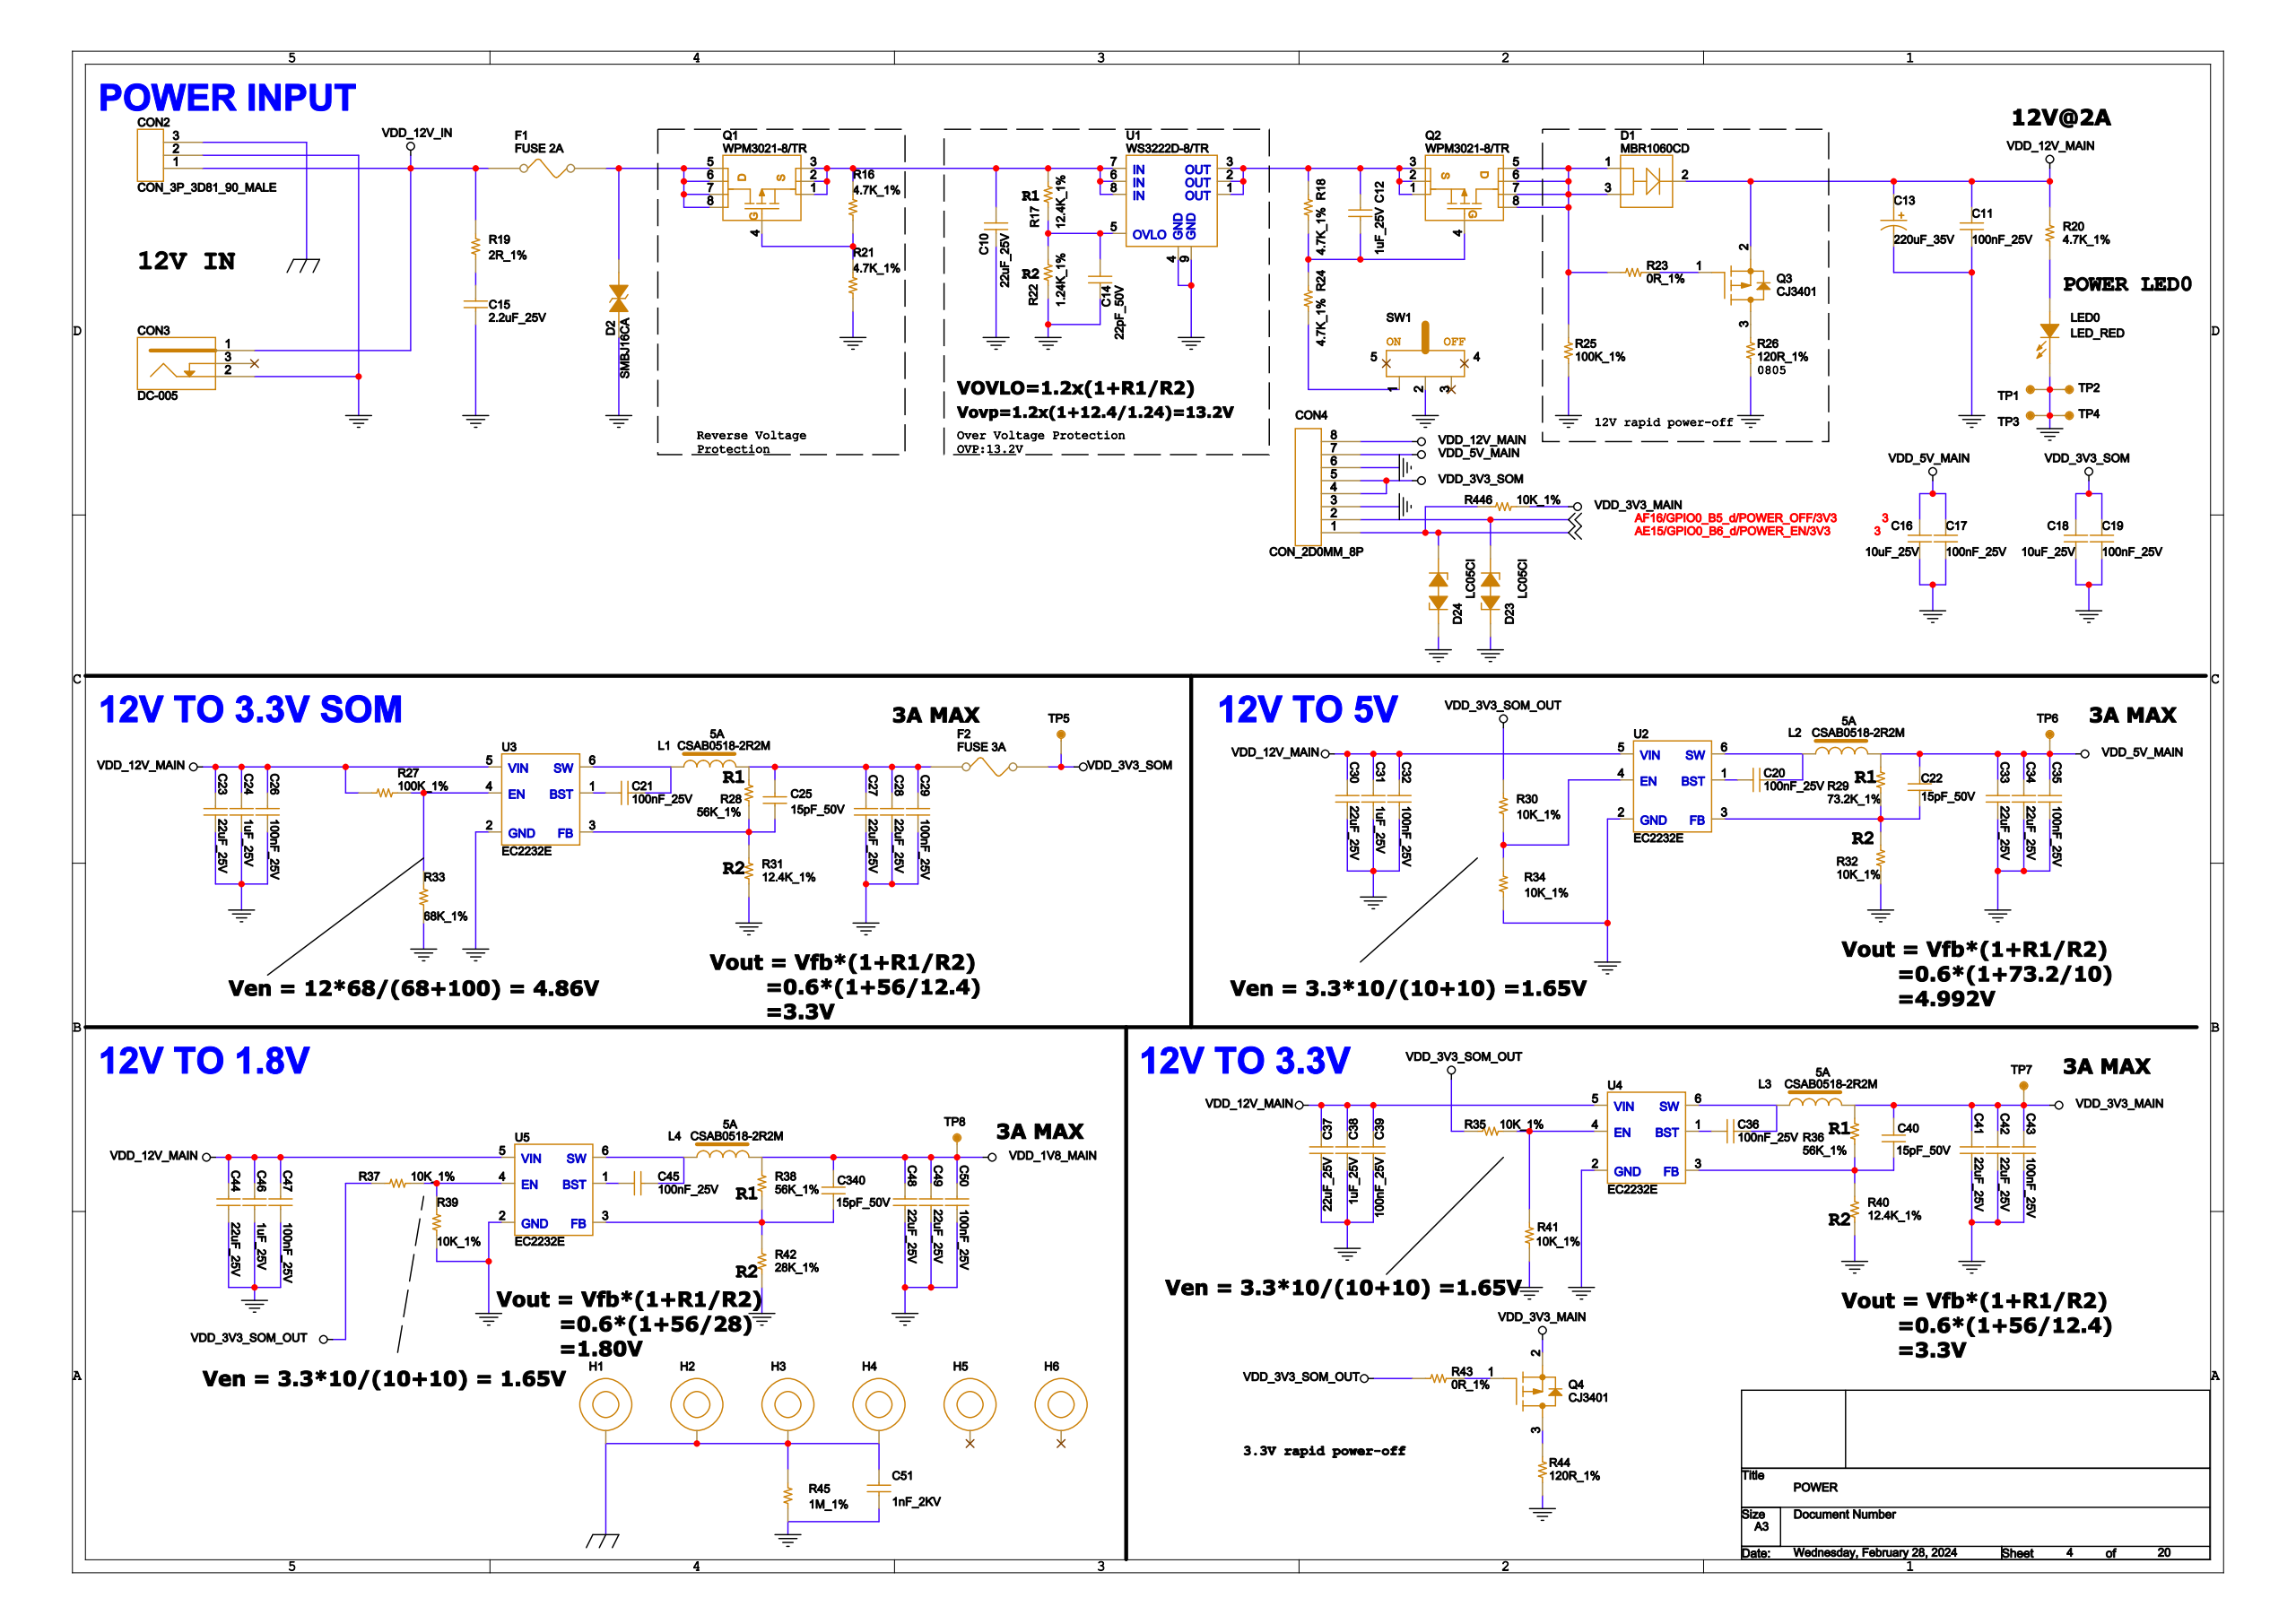Circuit board | Cadence Allegro | 1024 parts | 682 nets | one sheet of the schematic
Parts on this sheet (reference | value | footprint):
C10 | 22uF_25V | C0805
C11 | 100nF_25V | C0402
C12 | 1uF_25V | C0603
C13 | 220uF_35V | CAP_ALU_SMD_8X10D5
C14 | 22pF_50V | C0603
C15 | 2.2uF_25V | C1206
C16 | 10uF_25V | C0603
C17 | 100nF_25V | C0402
C18 | 10uF_25V | C0603
C19 | 100nF_25V | C0402
C20 | 100nF_25V | C0402
C21 | 100nF_25V | C0402
C22 | 15pF_50V | C0402
C23 | 22uF_25V | C0805
C24 | 1uF_25V | C0603
C25 | 15pF_50V | C0402
C26 | 100nF_25V | C0402
C27 | 22uF_25V | C0805
C28 | 22uF_25V | C0805
C29 | 100nF_25V | C0402
C30 | 22uF_25V | C0805
C31 | 1uF_25V | C0603
C32 | 100nF_25V | C0402
C33 | 22uF_25V | C0805
C34 | 22uF_25V | C0805
C35 | 100nF_25V | C0402
C36 | 100nF_25V | C0402
C37 | 22uF_25V | C0805
C38 | 1uF_25V | C0603
C39 | 100nF_25V | C0402
C40 | 15pF_50V | C0402
C41 | 22uF_25V | C0805
C42 | 22uF_25V | C0805
C43 | 100nF_25V | C0402
C44 | 22uF_25V | C0805
C45 | 100nF_25V | C0402
C46 | 1uF_25V | C0603
C47 | 100nF_25V | C0402
C48 | 22uF_25V | C0805
C49 | 22uF_25V | C0805
C50 | 100nF_25V | C0402
C51 | 1nF_2KV | C1210
C340 | 15pF_50V | C0402
CON2 | CON_3P_3D81_90_MALE | CON_3P_3D81_90_MALE_NEW
CON3 | 305-OT03SZD001 | CON_DC005_NEW
CON4 | CON_2D0MM_8P | DIP_CON_2D0MM_8P
D1 | MBR1060CD | TO-252
D2 | SMBJ16CA | SMB
D23 | LC05CI | SOD323_BI
D24 | LC05CI | SOD323_BI
F1 | FUSE 2A | F1206
F2 | FUSE 3A | F1206
H4 | HOLE | MHOLE_C200D125
L1 | CSAB0518-2R2M | SMD_CSAB0518
L2 | CSAB0518-2R2M | SMD_CSAB0518
L3 | CSAB0518-2R2M | SMD_CSAB0518
L4 | CSAB0518-2R2M | SMD_CSAB0518
Q1 | WPM3021-8/TR | PSOPSOP-8L
Q2 | WPM3021-8/TR | PSOPSOP-8L
Q3 | CJ3401 | SOT23-3
Q4 | CJ3401 | SOT23-3
R16 | 4.7K_1% | R0402
R17 | 12.4K_1% | R0402
R18 | 4.7K_1% | R0402
R19 | 2R_1% | R1210
R20 | 4.7K_1% | R0402
R21 | 4.7K_1% | R0402
R22 | 1.24K_1% | R0603
R23 | 0R_1% | R0402
R24 | 4.7K_1% | R0402
R25 | 100K_1% | R0402
R26 | 120R_1% | R0805
R27 | 100K_1% | R0402
R28 | 56K_1% | R0402
R29 | 73.2K_1% | R0402
R30 | 10K_1% | R0402
R31 | 12.4K_1% | R0402
R32 | 10K_1% | R0402
R33 | 68K_1% | R0402
R34 | 10K_1% | R0402
R35 | 10K_1% | R0402
R36 | 56K_1% | R0402
R37 | 10K_1% | R0402
R38 | 56K_1% | R0402
R39 | 10K_1% | R0402
R40 | 12.4K_1% | R0402
R41 | 10K_1% | R0402
R42 | 28K_1% | R0402
R43 | 0R_1% | R0402
R44 | 120R_1% | R0805
R45 | 1M_1% | R0603
R446 | 10K_1% | R0402
SW1 | SS-12D11L5 | SW-126_76
TP1 | Black Test Point | TP_DIP
TP2 | Black Test Point | TP_DIP
TP3 | Black Test Point | TP_DIP
TP4 | Black Test Point | TP_DIP
TP5 | SMT TP | TP30
TP6 | SMT TP | TP30
TP7 | SMT TP | TP30
TP8 | SMT TP | TP30
U1 | WS3222D-8/TR | DFN2X2-8L
U2 | EC2232E | SOT-23-6L
U3 | EC2232E | SOT-23-6L
U4 | EC2232E | SOT-23-6L
U5 | EC2232E | SOT-23-6L
Nets of these parts (net: part-pin ...):
GND: C10-2 C11-2 C13-2 C14-1 C15-2 C16-2 C17-2 C18-2 C19-2 C23-2 C24-2 C26-2 C27-2 C28-2 C29-2 C30-2 C31-2 C32-2 C33-2 C34-2 C35-2 C37-2 C38-2 C39-2 C41-2 C42-2 C43-2 C44-2 C46-2 C47-2 C48-2 C49-2 C50-2 C51-2 CON2-2 CON3-2 CON4-3 CON4-6 D2-1 D23-2 D24-2 R21-1 R22-2 R25-1 R26-2 R31-1 R32-1 R33-1 R34-1 R39-1 R40-1 R41-1 R42-1 R44-2 R45-2 SW1-2 TP1-1 TP2-1 TP3-1 TP4-1 U1-4 U1-9 U2-2 U3-2 U4-2 U5-2
VDD_5V_MAIN: C16-1 C17-1 C22-2 C33-1 C34-1 C35-1 CON4-7 L2-2 R29-2 TP6-1
VDD_1V8_MAIN: C48-1 C49-1 C50-1 C340-2 L4-2 R38-2 TP8-1
VDD_12V_IN: CON2-1 CON3-1 F1-1 R19-2
EGND: C51-1 CON2-3 H4-1 R45-1
VDD_3V3_MAIN: C40-2 C41-1 C42-1 C43-1 L3-2 Q4-2 R36-2 R446-1 TP7-1
N21580067: C22-1 R29-1 R32-2 U2-3
N21578849: C25-1 R28-1 R31-2 U3-3
N21578869: C25-2 C27-1 C28-1 C29-1 F2-1 L1-2 R28-2
N21581624: C340-1 R38-1 R42-2 U5-3
N21579453: C40-1 R36-1 R40-2 U4-3
VDD_3V3_SOM: C18-1 C19-1 CON4-4 CON4-5 F2-2 TP5-1
AF16/GPIO0_B5_D/POWER_OFF/3V3: CON4-2 D23-1
AE15/GPIO0_B6_D/POWER_EN/3V3: CON4-1 D24-1 R446-2
VDD_3V3_SOM_OUT: R30-2 R35-2 R37-1 R43-2
N21577998: D2-2 F1-2 Q1-5 Q1-6 Q1-7 Q1-8
VDD_12V_MAIN: C11-1 C13-1 C23-1 C24-1 C26-1 C30-1 C31-1 C32-1 C37-1 C38-1 C39-1 C44-1 C46-1 C47-1 CON4-8 D1-2 Q3-2 R20-1 R27-1 U2-5 U3-5 U4-5 U5-5
N21577837: R20-2
N21577996: Q1-4 R16-1 R21-2
N21577845: C10-1 Q1-1 Q1-2 Q1-3 R16-2 R17-1 U1-6 U1-7 U1-8
N21577994: C12-2 Q2-4 R18-1 R24-2
N21577869: C12-1 Q2-1 Q2-2 Q2-3 R18-2 U1-1 U1-2 U1-3
N21578066: R24-1 SW1-1
N21577906: C14-2 R17-2 R22-1 U1-5
N21577820: D1-1 D1-3 Q2-5 Q2-6 Q2-7 Q2-8 R23-2 R25-2
N21578757: R27-2 R33-2 U3-4
N21582083: Q4-1 R43-1
N21578248: Q3-1 R23-1
N21578352: C15-1 R19-1
N21581614: C45-1 U5-1
N21581612: C45-2 L4-1 U5-6
N21578843: C21-2 L1-1 U3-6
N21580045: C20-2 L2-1 U2-6
N21579439: C36-2 L3-1 U4-6
N21581706: R37-2 R39-2 U5-4
N21580047: C20-1 U2-1
N21578845: C21-1 U3-1
N21579441: C36-1 U4-1
N21582077: Q4-3 R44-1
N215782442: Q3-3 R26-1
N21580179: R30-1 R34-2 U2-4
N21579349: R35-1 R41-2 U4-4